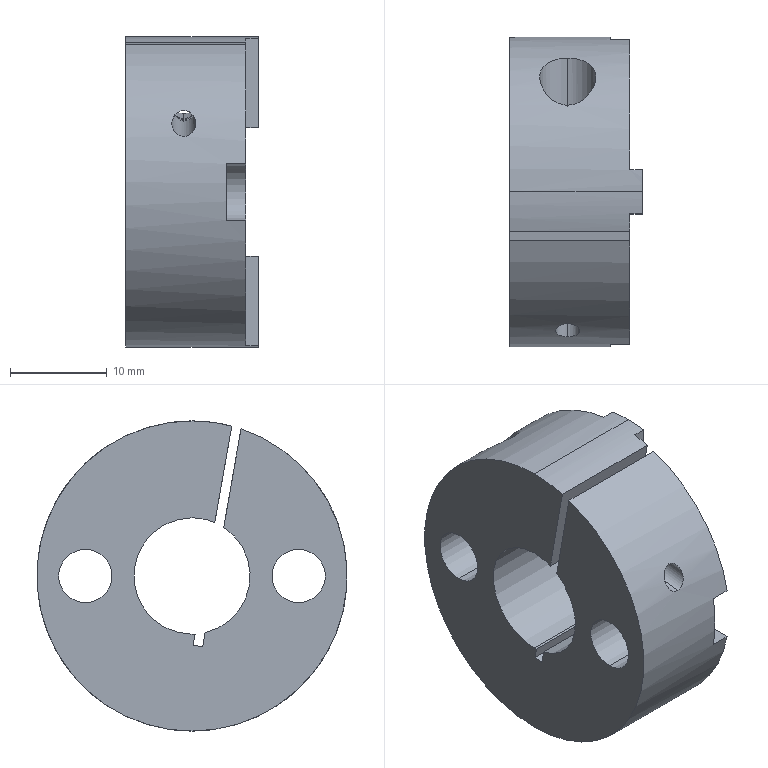Part | SolidWorks | features BaseBody 1, ICE 1 | 1 solid | 55 faces | box 13.7 x 32 x 32 mm | volume 7455 mm3 | cylinder 29 | plane 22 | cone 4 | commonest cylinder face diameters 2.459 x8 5.5 x4 12 x4 14 x4 32 x3 3.8 x2